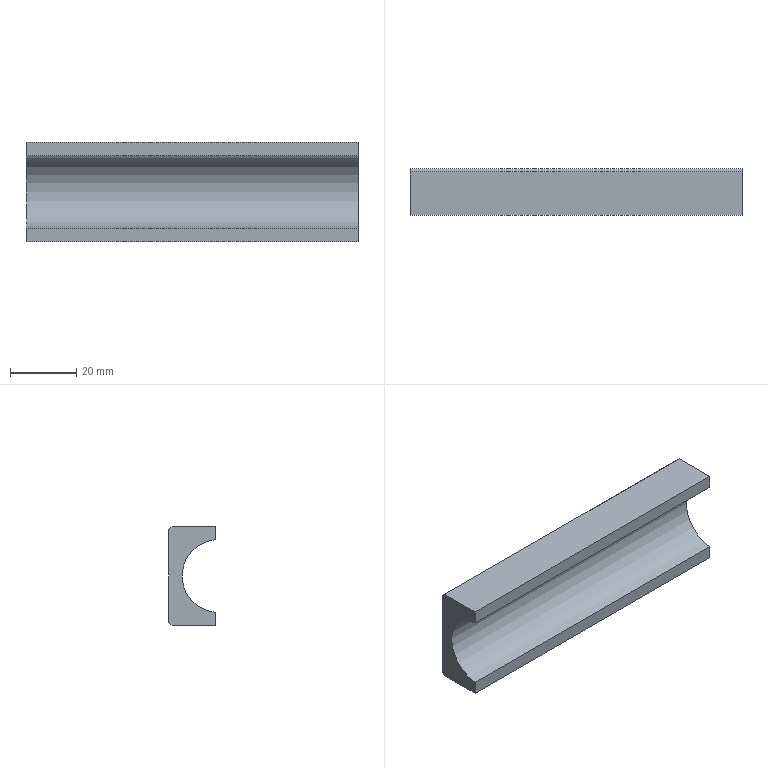Part | SolidWorks | features Chamfer 1, Extrusion 1, ICE 1 | 1 solid | 10 faces | box 100 x 14 x 30 mm | volume 25090 mm3 | plane 9 | cylinder 1 | commonest cylinder face diameters 22 x1
STEP:
#1=CARTESIAN_POINT('',(50.,-7.,4.046));
#2=VERTEX_POINT('',#1);
#3=CARTESIAN_POINT('',(50.,-7.,0.));
#4=VERTEX_POINT('',#3);
#5=CARTESIAN_POINT('',(50.,-7.,30.));
#6=DIRECTION('',(0.,0.,-1.));
#7=VECTOR('',#6,1000.);
#8=LINE('',#5,#7);
#9=EDGE_CURVE('',#2,#4,#8,.T.);
#10=ORIENTED_EDGE('',*,*,#9,.F.);
#11=CARTESIAN_POINT('',(-50.,-7.,4.046));
#12=VERTEX_POINT('',#11);
#13=CARTESIAN_POINT('',(50.,-7.,4.046));
#14=DIRECTION('',(-1.,0.,0.));
#15=VECTOR('',#14,1000.);
#16=LINE('',#13,#15);
#17=EDGE_CURVE('',#2,#12,#16,.T.);
#18=ORIENTED_EDGE('',*,*,#17,.T.);
#19=CARTESIAN_POINT('',(-50.,-7.,0.));
#20=VERTEX_POINT('',#19);
#21=CARTESIAN_POINT('',(-50.,-7.,30.));
#22=DIRECTION('',(0.,0.,-1.));
#23=VECTOR('',#22,1000.);
#24=LINE('',#21,#23);
#25=EDGE_CURVE('',#12,#20,#24,.T.);
#26=ORIENTED_EDGE('',*,*,#25,.T.);
#27=CARTESIAN_POINT('',(-50.,-7.,0.));
#28=DIRECTION('',(1.,0.,0.));
#29=VECTOR('',#28,1000.);
#30=LINE('',#27,#29);
#31=EDGE_CURVE('',#20,#4,#30,.T.);
#32=ORIENTED_EDGE('',*,*,#31,.T.);
#33=EDGE_LOOP('',(#10,#18,#26,#32));
#34=FACE_OUTER_BOUND('',#33,.T.);
#35=CARTESIAN_POINT('',(-50.,-7.,30.));
#36=DIRECTION('',(0.,1.,0.));
#37=DIRECTION('',(0.,0.,1.));
#38=AXIS2_PLACEMENT_3D('',#35,#36,#37);
#39=PLANE('',#38);
#40=ADVANCED_FACE('',(#34),#39,.F.);
#41=CARTESIAN_POINT('',(50.,6.,0.));
#42=VERTEX_POINT('',#41);
#43=CARTESIAN_POINT('',(50.,7.,0.));
#44=DIRECTION('',(0.,1.,0.));
#45=VECTOR('',#44,1000.);
#46=LINE('',#43,#45);
#47=EDGE_CURVE('',#4,#42,#46,.T.);
#48=ORIENTED_EDGE('',*,*,#47,.T.);
#49=CARTESIAN_POINT('',(50.,7.,1.));
#50=VERTEX_POINT('',#49);
#51=CARTESIAN_POINT('',(50.,7.,1.));
#52=DIRECTION('',(0.,0.7071,0.7071));
#53=VECTOR('',#52,1000.);
#54=LINE('',#51,#53);
#55=EDGE_CURVE('',#42,#50,#54,.T.);
#56=ORIENTED_EDGE('',*,*,#55,.T.);
#57=CARTESIAN_POINT('',(50.,7.,29.));
#58=VERTEX_POINT('',#57);
#59=CARTESIAN_POINT('',(50.,7.,30.));
#60=DIRECTION('',(0.,0.,-1.));
#61=VECTOR('',#60,1000.);
#62=LINE('',#59,#61);
#63=EDGE_CURVE('',#58,#50,#62,.T.);
#64=ORIENTED_EDGE('',*,*,#63,.F.);
#65=CARTESIAN_POINT('',(50.,6.,30.));
#66=VERTEX_POINT('',#65);
#67=CARTESIAN_POINT('',(50.,6.,30.));
#68=DIRECTION('',(0.,-0.7071,0.7071));
#69=VECTOR('',#68,1000.);
#70=LINE('',#67,#69);
#71=EDGE_CURVE('',#58,#66,#70,.T.);
#72=ORIENTED_EDGE('',*,*,#71,.T.);
#73=CARTESIAN_POINT('',(50.,-7.,30.));
#74=VERTEX_POINT('',#73);
#75=CARTESIAN_POINT('',(50.,7.,30.));
#76=DIRECTION('',(0.,1.,0.));
#77=VECTOR('',#76,1000.);
#78=LINE('',#75,#77);
#79=EDGE_CURVE('',#74,#66,#78,.T.);
#80=ORIENTED_EDGE('',*,*,#79,.F.);
#81=CARTESIAN_POINT('',(50.,-7.,25.954));
#82=VERTEX_POINT('',#81);
#83=CARTESIAN_POINT('',(50.,-7.,30.));
#84=DIRECTION('',(0.,0.,-1.));
#85=VECTOR('',#84,1000.);
#86=LINE('',#83,#85);
#87=EDGE_CURVE('',#74,#82,#86,.T.);
#88=ORIENTED_EDGE('',*,*,#87,.T.);
#89=CARTESIAN_POINT('',(50.,-8.,15.));
#90=DIRECTION('',(-1.,0.,0.));
#91=DIRECTION('',(0.,-1.,0.));
#92=AXIS2_PLACEMENT_3D('',#89,#90,#91);
#93=CIRCLE('',#92,11.);
#94=EDGE_CURVE('',#82,#2,#93,.T.);
#95=ORIENTED_EDGE('',*,*,#94,.T.);
#96=ORIENTED_EDGE('',*,*,#9,.T.);
#97=EDGE_LOOP('',(#48,#56,#64,#72,#80,#88,#95,#96));
#98=FACE_OUTER_BOUND('',#97,.T.);
#99=CARTESIAN_POINT('',(50.,7.,30.));
#100=DIRECTION('',(-1.,0.,0.));
#101=DIRECTION('',(0.,0.,1.));
#102=AXIS2_PLACEMENT_3D('',#99,#100,#101);
#103=PLANE('',#102);
#104=ADVANCED_FACE('',(#98),#103,.F.);
#105=ORIENTED_EDGE('',*,*,#63,.T.);
#106=CARTESIAN_POINT('',(-50.,7.,1.));
#107=VERTEX_POINT('',#106);
#108=CARTESIAN_POINT('',(-50.,7.,1.));
#109=DIRECTION('',(-1.,0.,0.));
#110=VECTOR('',#109,1000.);
#111=LINE('',#108,#110);
#112=EDGE_CURVE('',#50,#107,#111,.T.);
#113=ORIENTED_EDGE('',*,*,#112,.T.);
#114=CARTESIAN_POINT('',(-50.,7.,29.));
#115=VERTEX_POINT('',#114);
#116=CARTESIAN_POINT('',(-50.,7.,30.));
#117=DIRECTION('',(0.,0.,-1.));
#118=VECTOR('',#117,1000.);
#119=LINE('',#116,#118);
#120=EDGE_CURVE('',#115,#107,#119,.T.);
#121=ORIENTED_EDGE('',*,*,#120,.F.);
#122=CARTESIAN_POINT('',(50.,7.,29.));
#123=DIRECTION('',(1.,0.,0.));
#124=VECTOR('',#123,1000.);
#125=LINE('',#122,#124);
#126=EDGE_CURVE('',#115,#58,#125,.T.);
#127=ORIENTED_EDGE('',*,*,#126,.T.);
#128=EDGE_LOOP('',(#105,#113,#121,#127));
#129=FACE_OUTER_BOUND('',#128,.T.);
#130=CARTESIAN_POINT('',(-50.,7.,30.));
#131=DIRECTION('',(0.,-1.,0.));
#132=DIRECTION('',(0.,0.,-1.));
#133=AXIS2_PLACEMENT_3D('',#130,#131,#132);
#134=PLANE('',#133);
#135=ADVANCED_FACE('',(#129),#134,.F.);
#136=ORIENTED_EDGE('',*,*,#120,.T.);
#137=CARTESIAN_POINT('',(-50.,6.,0.));
#138=VERTEX_POINT('',#137);
#139=CARTESIAN_POINT('',(-50.,7.,1.));
#140=DIRECTION('',(0.,-0.7071,-0.7071));
#141=VECTOR('',#140,1000.);
#142=LINE('',#139,#141);
#143=EDGE_CURVE('',#107,#138,#142,.T.);
#144=ORIENTED_EDGE('',*,*,#143,.T.);
#145=CARTESIAN_POINT('',(-50.,7.,0.));
#146=DIRECTION('',(0.,-1.,0.));
#147=VECTOR('',#146,1000.);
#148=LINE('',#145,#147);
#149=EDGE_CURVE('',#138,#20,#148,.T.);
#150=ORIENTED_EDGE('',*,*,#149,.T.);
#151=ORIENTED_EDGE('',*,*,#25,.F.);
#152=CARTESIAN_POINT('',(-50.,-7.,25.954));
#153=VERTEX_POINT('',#152);
#154=CARTESIAN_POINT('',(-50.,-8.,15.));
#155=DIRECTION('',(-1.,0.,0.));
#156=DIRECTION('',(0.,-1.,0.));
#157=AXIS2_PLACEMENT_3D('',#154,#155,#156);
#158=CIRCLE('',#157,11.);
#159=EDGE_CURVE('',#153,#12,#158,.T.);
#160=ORIENTED_EDGE('',*,*,#159,.F.);
#161=CARTESIAN_POINT('',(-50.,-7.,30.));
#162=VERTEX_POINT('',#161);
#163=CARTESIAN_POINT('',(-50.,-7.,30.));
#164=DIRECTION('',(0.,0.,-1.));
#165=VECTOR('',#164,1000.);
#166=LINE('',#163,#165);
#167=EDGE_CURVE('',#162,#153,#166,.T.);
#168=ORIENTED_EDGE('',*,*,#167,.F.);
#169=CARTESIAN_POINT('',(-50.,6.,30.));
#170=VERTEX_POINT('',#169);
#171=CARTESIAN_POINT('',(-50.,7.,30.));
#172=DIRECTION('',(0.,-1.,0.));
#173=VECTOR('',#172,1000.);
#174=LINE('',#171,#173);
#175=EDGE_CURVE('',#170,#162,#174,.T.);
#176=ORIENTED_EDGE('',*,*,#175,.F.);
#177=CARTESIAN_POINT('',(-50.,6.,30.));
#178=DIRECTION('',(0.,0.7071,-0.7071));
#179=VECTOR('',#178,1000.);
#180=LINE('',#177,#179);
#181=EDGE_CURVE('',#170,#115,#180,.T.);
#182=ORIENTED_EDGE('',*,*,#181,.T.);
#183=EDGE_LOOP('',(#136,#144,#150,#151,#160,#168,#176,#182));
#184=FACE_OUTER_BOUND('',#183,.T.);
#185=CARTESIAN_POINT('',(-50.,7.,30.));
#186=DIRECTION('',(1.,0.,0.));
#187=DIRECTION('',(0.,0.,-1.));
#188=AXIS2_PLACEMENT_3D('',#185,#186,#187);
#189=PLANE('',#188);
#190=ADVANCED_FACE('',(#184),#189,.F.);
#191=ORIENTED_EDGE('',*,*,#167,.T.);
#192=CARTESIAN_POINT('',(50.,-7.,25.954));
#193=DIRECTION('',(1.,0.,0.));
#194=VECTOR('',#193,1000.);
#195=LINE('',#192,#194);
#196=EDGE_CURVE('',#153,#82,#195,.T.);
#197=ORIENTED_EDGE('',*,*,#196,.T.);
#198=ORIENTED_EDGE('',*,*,#87,.F.);
#199=CARTESIAN_POINT('',(-50.,-7.,30.));
#200=DIRECTION('',(1.,0.,0.));
#201=VECTOR('',#200,1000.);
#202=LINE('',#199,#201);
#203=EDGE_CURVE('',#162,#74,#202,.T.);
#204=ORIENTED_EDGE('',*,*,#203,.F.);
#205=EDGE_LOOP('',(#191,#197,#198,#204));
#206=FACE_OUTER_BOUND('',#205,.T.);
#207=CARTESIAN_POINT('',(-50.,-7.,30.));
#208=DIRECTION('',(0.,1.,0.));
#209=DIRECTION('',(0.,0.,1.));
#210=AXIS2_PLACEMENT_3D('',#207,#208,#209);
#211=PLANE('',#210);
#212=ADVANCED_FACE('',(#206),#211,.F.);
#213=ORIENTED_EDGE('',*,*,#79,.T.);
#214=CARTESIAN_POINT('',(-50.,6.,30.));
#215=DIRECTION('',(-1.,0.,0.));
#216=VECTOR('',#215,1000.);
#217=LINE('',#214,#216);
#218=EDGE_CURVE('',#66,#170,#217,.T.);
#219=ORIENTED_EDGE('',*,*,#218,.T.);
#220=ORIENTED_EDGE('',*,*,#175,.T.);
#221=ORIENTED_EDGE('',*,*,#203,.T.);
#222=EDGE_LOOP('',(#213,#219,#220,#221));
#223=FACE_OUTER_BOUND('',#222,.T.);
#224=CARTESIAN_POINT('',(0.,0.,30.));
#225=DIRECTION('',(0.,0.,1.));
#226=DIRECTION('',(1.,0.,0.));
#227=AXIS2_PLACEMENT_3D('',#224,#225,#226);
#228=PLANE('',#227);
#229=ADVANCED_FACE('',(#223),#228,.T.);
#230=ORIENTED_EDGE('',*,*,#149,.F.);
#231=CARTESIAN_POINT('',(0.,6.,0.));
#232=DIRECTION('',(1.,0.,0.));
#233=VECTOR('',#232,1000.);
#234=LINE('',#231,#233);
#235=EDGE_CURVE('',#138,#42,#234,.T.);
#236=ORIENTED_EDGE('',*,*,#235,.T.);
#237=ORIENTED_EDGE('',*,*,#47,.F.);
#238=ORIENTED_EDGE('',*,*,#31,.F.);
#239=EDGE_LOOP('',(#230,#236,#237,#238));
#240=FACE_OUTER_BOUND('',#239,.T.);
#241=CARTESIAN_POINT('',(0.,0.,0.));
#242=DIRECTION('',(0.,0.,1.));
#243=DIRECTION('',(1.,0.,0.));
#244=AXIS2_PLACEMENT_3D('',#241,#242,#243);
#245=PLANE('',#244);
#246=ADVANCED_FACE('',(#240),#245,.F.);
#247=ORIENTED_EDGE('',*,*,#94,.F.);
#248=ORIENTED_EDGE('',*,*,#196,.F.);
#249=ORIENTED_EDGE('',*,*,#159,.T.);
#250=ORIENTED_EDGE('',*,*,#17,.F.);
#251=EDGE_LOOP('',(#247,#248,#249,#250));
#252=FACE_OUTER_BOUND('',#251,.T.);
#253=CARTESIAN_POINT('',(50.,-8.,15.));
#254=DIRECTION('',(-1.,0.,0.));
#255=DIRECTION('',(0.,-1.,0.));
#256=AXIS2_PLACEMENT_3D('',#253,#254,#255);
#257=CYLINDRICAL_SURFACE('',#256,11.);
#258=ADVANCED_FACE('',(#252),#257,.F.);
#259=ORIENTED_EDGE('',*,*,#55,.F.);
#260=ORIENTED_EDGE('',*,*,#235,.F.);
#261=ORIENTED_EDGE('',*,*,#143,.F.);
#262=ORIENTED_EDGE('',*,*,#112,.F.);
#263=EDGE_LOOP('',(#259,#260,#261,#262));
#264=FACE_OUTER_BOUND('',#263,.T.);
#265=CARTESIAN_POINT('',(-50.,7.,1.));
#266=DIRECTION('',(0.,-0.7071,0.7071));
#267=DIRECTION('',(-1.,0.,0.));
#268=AXIS2_PLACEMENT_3D('',#265,#266,#267);
#269=PLANE('',#268);
#270=ADVANCED_FACE('',(#264),#269,.F.);
#271=ORIENTED_EDGE('',*,*,#71,.F.);
#272=ORIENTED_EDGE('',*,*,#126,.F.);
#273=ORIENTED_EDGE('',*,*,#181,.F.);
#274=ORIENTED_EDGE('',*,*,#218,.F.);
#275=EDGE_LOOP('',(#271,#272,#273,#274));
#276=FACE_OUTER_BOUND('',#275,.T.);
#277=CARTESIAN_POINT('',(0.,6.,30.));
#278=DIRECTION('',(0.,0.7071,0.7071));
#279=DIRECTION('',(1.,0.,0.));
#280=AXIS2_PLACEMENT_3D('',#277,#278,#279);
#281=PLANE('',#280);
#282=ADVANCED_FACE('',(#276),#281,.T.);
#283=CLOSED_SHELL('',(#40,#104,#135,#190,#212,#229,#246,#258,#270,#282));
#284=MANIFOLD_SOLID_BREP('',#283);
#285=CARTESIAN_POINT('',(0.,0.,0.));
#286=DIRECTION('',(0.,0.,1.));
#287=DIRECTION('',(1.,0.,0.));
#288=AXIS2_PLACEMENT_3D('',#285,#286,#287);
#289=(LENGTH_UNIT()NAMED_UNIT(*)SI_UNIT(.MILLI.,.METRE.));
#290=UNCERTAINTY_MEASURE_WITH_UNIT(LENGTH_MEASURE(0.00001),#289,'','');
#291=(NAMED_UNIT(*)PLANE_ANGLE_UNIT()SI_UNIT($,.RADIAN.));
#292=(NAMED_UNIT(*)SI_UNIT($,.STERADIAN.)SOLID_ANGLE_UNIT());
#293=(GEOMETRIC_REPRESENTATION_CONTEXT(3)GLOBAL_UNCERTAINTY_ASSIGNED_CONTEXT((#290))GLOBAL_UNIT_ASSIGNED_CONTEXT((#289,#291,#292))REPRESENTATION_CONTEXT('',''));
#294=ADVANCED_BREP_SHAPE_REPRESENTATION('',(#284,#288),#293);